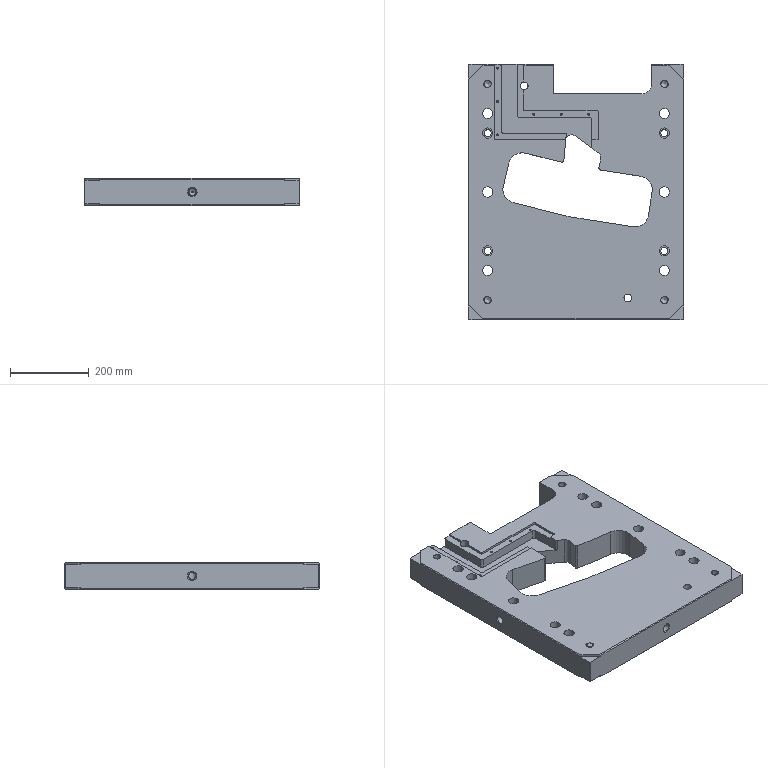Part | STEP file | P011002A003-000 | 1 solid | 807 faces | box 550 x 650 x 70 mm | volume 18968143 mm3 | plane 536 | other 93 | cylinder 91 | cone 87 | commonest cylinder face diameters 5 x12 10 x10 26 x10 20 x9 4.167 x8 4.983 x8